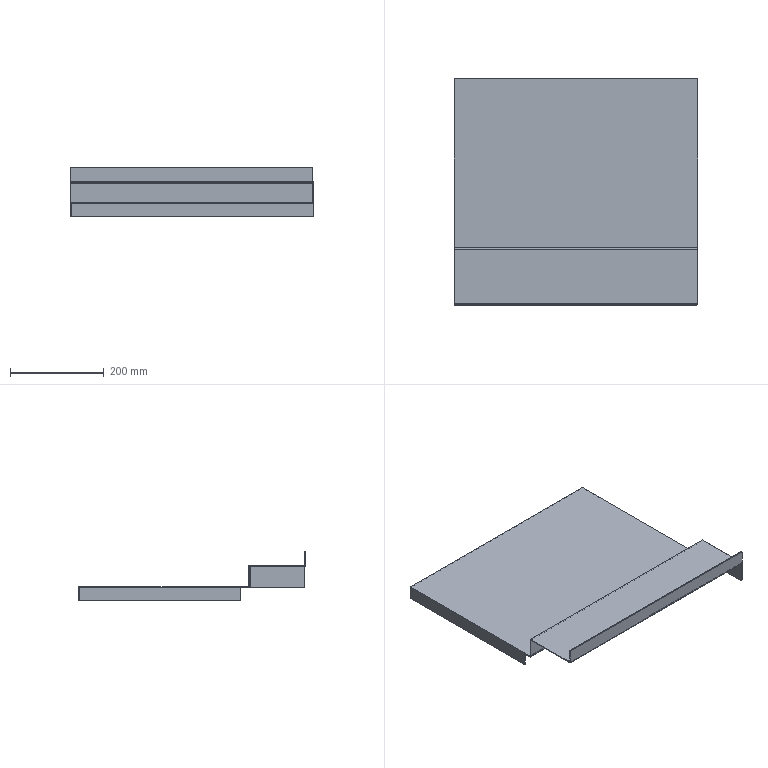Part | STEP file | 11-GYJJ-012-q111 | 1 solid | 31 faces | box 521 x 485 x 105 mm | volume 642321 mm3 | plane 21 | cylinder 10 | commonest cylinder face diameters 4 x10
STEP:
#1=CARTESIAN_POINT('',(258.5,-300.5,45.));
#2=VERTEX_POINT('',#1);
#3=CARTESIAN_POINT('',(258.5,-184.5,45.));
#4=VERTEX_POINT('',#3);
#5=CARTESIAN_POINT('',(258.5,-184.5,45.));
#6=DIRECTION('',(0.,1.,0.));
#7=VECTOR('',#6,1000.);
#8=LINE('',#5,#7);
#9=EDGE_CURVE('',#2,#4,#8,.T.);
#10=ORIENTED_EDGE('',*,*,#9,.F.);
#11=CARTESIAN_POINT('',(-260.5,-300.5,45.));
#12=VERTEX_POINT('',#11);
#13=CARTESIAN_POINT('',(-260.5,-300.5,45.));
#14=DIRECTION('',(-1.,0.,0.));
#15=VECTOR('',#14,1000.);
#16=LINE('',#13,#15);
#17=EDGE_CURVE('',#2,#12,#16,.T.);
#18=ORIENTED_EDGE('',*,*,#17,.T.);
#19=CARTESIAN_POINT('',(-260.5,-184.5,45.));
#20=VERTEX_POINT('',#19);
#21=CARTESIAN_POINT('',(-260.5,-302.5,45.));
#22=DIRECTION('',(0.,1.,0.));
#23=VECTOR('',#22,1000.);
#24=LINE('',#21,#23);
#25=EDGE_CURVE('',#12,#20,#24,.T.);
#26=ORIENTED_EDGE('',*,*,#25,.T.);
#27=CARTESIAN_POINT('',(260.5,-184.5,45.));
#28=DIRECTION('',(1.,0.,0.));
#29=VECTOR('',#28,1000.);
#30=LINE('',#27,#29);
#31=EDGE_CURVE('',#20,#4,#30,.T.);
#32=ORIENTED_EDGE('',*,*,#31,.T.);
#33=EDGE_LOOP('',(#10,#18,#26,#32));
#34=FACE_OUTER_BOUND('',#33,.T.);
#35=CARTESIAN_POINT('',(-260.5,-302.5,45.));
#36=DIRECTION('',(0.,0.,1.));
#37=DIRECTION('',(1.,0.,0.));
#38=AXIS2_PLACEMENT_3D('',#35,#36,#37);
#39=PLANE('',#38);
#40=ADVANCED_FACE('',(#34),#39,.F.);
#41=CARTESIAN_POINT('',(-260.5,-182.5,47.));
#42=VERTEX_POINT('',#41);
#43=CARTESIAN_POINT('',(-260.5,-298.5,47.));
#44=VERTEX_POINT('',#43);
#45=CARTESIAN_POINT('',(-260.5,-182.5,47.));
#46=DIRECTION('',(0.,-1.,0.));
#47=VECTOR('',#46,1000.);
#48=LINE('',#45,#47);
#49=EDGE_CURVE('',#42,#44,#48,.T.);
#50=ORIENTED_EDGE('',*,*,#49,.T.);
#51=CARTESIAN_POINT('',(258.5,-298.5,47.));
#52=VERTEX_POINT('',#51);
#53=CARTESIAN_POINT('',(260.5,-298.5,47.));
#54=DIRECTION('',(1.,0.,0.));
#55=VECTOR('',#54,1000.);
#56=LINE('',#53,#55);
#57=EDGE_CURVE('',#44,#52,#56,.T.);
#58=ORIENTED_EDGE('',*,*,#57,.T.);
#59=CARTESIAN_POINT('',(258.5,-300.5,47.));
#60=VERTEX_POINT('',#59);
#61=CARTESIAN_POINT('',(258.5,-298.5,47.));
#62=DIRECTION('',(0.,1.,0.));
#63=VECTOR('',#62,1000.);
#64=LINE('',#61,#63);
#65=EDGE_CURVE('',#60,#52,#64,.T.);
#66=ORIENTED_EDGE('',*,*,#65,.F.);
#67=CARTESIAN_POINT('',(260.5,-300.5,47.));
#68=VERTEX_POINT('',#67);
#69=CARTESIAN_POINT('',(255.672,-300.5,47.));
#70=DIRECTION('',(1.,0.,0.));
#71=VECTOR('',#70,1000.);
#72=LINE('',#69,#71);
#73=EDGE_CURVE('',#60,#68,#72,.T.);
#74=ORIENTED_EDGE('',*,*,#73,.T.);
#75=CARTESIAN_POINT('',(260.5,-182.5,47.));
#76=VERTEX_POINT('',#75);
#77=CARTESIAN_POINT('',(260.5,-182.5,47.));
#78=DIRECTION('',(0.,1.,0.));
#79=VECTOR('',#78,1000.);
#80=LINE('',#77,#79);
#81=EDGE_CURVE('',#68,#76,#80,.T.);
#82=ORIENTED_EDGE('',*,*,#81,.T.);
#83=CARTESIAN_POINT('',(0.,-182.5,47.));
#84=DIRECTION('',(-1.,0.,0.));
#85=VECTOR('',#84,1000.);
#86=LINE('',#83,#85);
#87=EDGE_CURVE('',#76,#42,#86,.T.);
#88=ORIENTED_EDGE('',*,*,#87,.T.);
#89=EDGE_LOOP('',(#50,#58,#66,#74,#82,#88));
#90=FACE_OUTER_BOUND('',#89,.T.);
#91=CARTESIAN_POINT('',(0.,0.,47.));
#92=DIRECTION('',(0.,0.,-1.));
#93=DIRECTION('',(-1.,0.,0.));
#94=AXIS2_PLACEMENT_3D('',#91,#92,#93);
#95=PLANE('',#94);
#96=ADVANCED_FACE('',(#90),#95,.F.);
#97=CARTESIAN_POINT('',(260.5,-182.5,43.));
#98=VERTEX_POINT('',#97);
#99=CARTESIAN_POINT('',(260.5,-182.5,2.));
#100=VERTEX_POINT('',#99);
#101=CARTESIAN_POINT('',(260.5,-182.5,2.));
#102=DIRECTION('',(0.,0.,-1.));
#103=VECTOR('',#102,1000.);
#104=LINE('',#101,#103);
#105=EDGE_CURVE('',#98,#100,#104,.T.);
#106=ORIENTED_EDGE('',*,*,#105,.F.);
#107=CARTESIAN_POINT('',(-260.5,-182.5,43.));
#108=VERTEX_POINT('',#107);
#109=CARTESIAN_POINT('',(-260.5,-182.5,43.));
#110=DIRECTION('',(-1.,0.,0.));
#111=VECTOR('',#110,1000.);
#112=LINE('',#109,#111);
#113=EDGE_CURVE('',#98,#108,#112,.T.);
#114=ORIENTED_EDGE('',*,*,#113,.T.);
#115=CARTESIAN_POINT('',(-260.5,-182.5,2.));
#116=VERTEX_POINT('',#115);
#117=CARTESIAN_POINT('',(-260.5,-182.5,2.));
#118=DIRECTION('',(0.,0.,-1.));
#119=VECTOR('',#118,1000.);
#120=LINE('',#117,#119);
#121=EDGE_CURVE('',#108,#116,#120,.T.);
#122=ORIENTED_EDGE('',*,*,#121,.T.);
#123=CARTESIAN_POINT('',(-260.5,-182.5,2.));
#124=DIRECTION('',(1.,0.,0.));
#125=VECTOR('',#124,1000.);
#126=LINE('',#123,#125);
#127=EDGE_CURVE('',#116,#100,#126,.T.);
#128=ORIENTED_EDGE('',*,*,#127,.T.);
#129=EDGE_LOOP('',(#106,#114,#122,#128));
#130=FACE_OUTER_BOUND('',#129,.T.);
#131=CARTESIAN_POINT('',(-260.5,-182.5,2.));
#132=DIRECTION('',(0.,1.,0.));
#133=DIRECTION('',(0.,0.,1.));
#134=AXIS2_PLACEMENT_3D('',#131,#132,#133);
#135=PLANE('',#134);
#136=ADVANCED_FACE('',(#130),#135,.F.);
#137=CARTESIAN_POINT('',(260.5,-180.5,0.));
#138=VERTEX_POINT('',#137);
#139=CARTESIAN_POINT('',(260.5,180.5,0.));
#140=VERTEX_POINT('',#139);
#141=CARTESIAN_POINT('',(260.5,182.5,0.));
#142=DIRECTION('',(0.,1.,0.));
#143=VECTOR('',#142,1000.);
#144=LINE('',#141,#143);
#145=EDGE_CURVE('',#138,#140,#144,.T.);
#146=ORIENTED_EDGE('',*,*,#145,.F.);
#147=CARTESIAN_POINT('',(-260.5,-180.5,0.));
#148=VERTEX_POINT('',#147);
#149=CARTESIAN_POINT('',(0.,-180.5,0.));
#150=DIRECTION('',(-1.,0.,0.));
#151=VECTOR('',#150,1000.);
#152=LINE('',#149,#151);
#153=EDGE_CURVE('',#138,#148,#152,.T.);
#154=ORIENTED_EDGE('',*,*,#153,.T.);
#155=CARTESIAN_POINT('',(-260.5,-164.5,0.));
#156=VERTEX_POINT('',#155);
#157=CARTESIAN_POINT('',(-260.5,182.5,0.));
#158=DIRECTION('',(0.,-1.,0.));
#159=VECTOR('',#158,1000.);
#160=LINE('',#157,#159);
#161=EDGE_CURVE('',#156,#148,#160,.T.);
#162=ORIENTED_EDGE('',*,*,#161,.F.);
#163=CARTESIAN_POINT('',(-258.5,-164.5,0.));
#164=VERTEX_POINT('',#163);
#165=CARTESIAN_POINT('',(-260.5,-164.5,0.));
#166=DIRECTION('',(-1.,0.,0.));
#167=VECTOR('',#166,1000.);
#168=LINE('',#165,#167);
#169=EDGE_CURVE('',#164,#156,#168,.T.);
#170=ORIENTED_EDGE('',*,*,#169,.F.);
#171=CARTESIAN_POINT('',(-258.5,180.5,0.));
#172=VERTEX_POINT('',#171);
#173=CARTESIAN_POINT('',(-258.5,180.5,0.));
#174=DIRECTION('',(0.,-1.,0.));
#175=VECTOR('',#174,1000.);
#176=LINE('',#173,#175);
#177=EDGE_CURVE('',#172,#164,#176,.T.);
#178=ORIENTED_EDGE('',*,*,#177,.F.);
#179=CARTESIAN_POINT('',(260.5,180.5,0.));
#180=DIRECTION('',(-1.,0.,0.));
#181=VECTOR('',#180,1000.);
#182=LINE('',#179,#181);
#183=EDGE_CURVE('',#140,#172,#182,.T.);
#184=ORIENTED_EDGE('',*,*,#183,.F.);
#185=EDGE_LOOP('',(#146,#154,#162,#170,#178,#184));
#186=FACE_OUTER_BOUND('',#185,.T.);
#187=CARTESIAN_POINT('',(0.,0.,0.));
#188=DIRECTION('',(0.,0.,1.));
#189=DIRECTION('',(1.,0.,0.));
#190=AXIS2_PLACEMENT_3D('',#187,#188,#189);
#191=PLANE('',#190);
#192=ADVANCED_FACE('',(#186),#191,.F.);
#193=CARTESIAN_POINT('',(-258.5,180.5,-28.));
#194=VERTEX_POINT('',#193);
#195=CARTESIAN_POINT('',(-258.5,180.5,-28.));
#196=DIRECTION('',(0.,0.,1.));
#197=VECTOR('',#196,1000.);
#198=LINE('',#195,#197);
#199=EDGE_CURVE('',#194,#172,#198,.T.);
#200=ORIENTED_EDGE('',*,*,#199,.F.);
#201=CARTESIAN_POINT('',(260.5,180.5,-28.));
#202=VERTEX_POINT('',#201);
#203=CARTESIAN_POINT('',(260.5,180.5,-28.));
#204=DIRECTION('',(-1.,0.,0.));
#205=VECTOR('',#204,1000.);
#206=LINE('',#203,#205);
#207=EDGE_CURVE('',#202,#194,#206,.T.);
#208=ORIENTED_EDGE('',*,*,#207,.F.);
#209=CARTESIAN_POINT('',(260.5,180.5,-28.));
#210=DIRECTION('',(0.,0.,1.));
#211=VECTOR('',#210,1000.);
#212=LINE('',#209,#211);
#213=EDGE_CURVE('',#202,#140,#212,.T.);
#214=ORIENTED_EDGE('',*,*,#213,.T.);
#215=ORIENTED_EDGE('',*,*,#183,.T.);
#216=EDGE_LOOP('',(#200,#208,#214,#215));
#217=FACE_OUTER_BOUND('',#216,.T.);
#218=CARTESIAN_POINT('',(260.5,180.5,-28.));
#219=DIRECTION('',(0.,1.,0.));
#220=DIRECTION('',(-1.,0.,0.));
#221=AXIS2_PLACEMENT_3D('',#218,#219,#220);
#222=PLANE('',#221);
#223=ADVANCED_FACE('',(#217),#222,.F.);
#224=CARTESIAN_POINT('',(260.5,-298.5,0.));
#225=VERTEX_POINT('',#224);
#226=CARTESIAN_POINT('',(260.5,-186.5,0.));
#227=VERTEX_POINT('',#226);
#228=CARTESIAN_POINT('',(260.5,-184.5,0.));
#229=DIRECTION('',(0.,1.,0.));
#230=VECTOR('',#229,1000.);
#231=LINE('',#228,#230);
#232=EDGE_CURVE('',#225,#227,#231,.T.);
#233=ORIENTED_EDGE('',*,*,#232,.T.);
#234=CARTESIAN_POINT('',(260.5,-184.5,2.));
#235=VERTEX_POINT('',#234);
#236=CARTESIAN_POINT('',(260.5,-186.5,2.));
#237=DIRECTION('',(1.,0.,0.));
#238=DIRECTION('',(0.,0.,1.));
#239=AXIS2_PLACEMENT_3D('',#236,#237,#238);
#240=CIRCLE('',#239,2.);
#241=EDGE_CURVE('',#227,#235,#240,.T.);
#242=ORIENTED_EDGE('',*,*,#241,.T.);
#243=CARTESIAN_POINT('',(260.5,-184.5,45.));
#244=VERTEX_POINT('',#243);
#245=CARTESIAN_POINT('',(260.5,-184.5,-116.017));
#246=DIRECTION('',(0.,0.,1.));
#247=VECTOR('',#246,1000.);
#248=LINE('',#245,#247);
#249=EDGE_CURVE('',#235,#244,#248,.T.);
#250=ORIENTED_EDGE('',*,*,#249,.T.);
#251=CARTESIAN_POINT('',(260.5,-184.5,43.));
#252=DIRECTION('',(-1.,0.,0.));
#253=DIRECTION('',(0.,0.,1.));
#254=AXIS2_PLACEMENT_3D('',#251,#252,#253);
#255=CIRCLE('',#254,2.);
#256=EDGE_CURVE('',#244,#98,#255,.T.);
#257=ORIENTED_EDGE('',*,*,#256,.T.);
#258=ORIENTED_EDGE('',*,*,#105,.T.);
#259=CARTESIAN_POINT('',(260.5,-180.5,2.));
#260=DIRECTION('',(1.,0.,0.));
#261=DIRECTION('',(0.,0.,1.));
#262=AXIS2_PLACEMENT_3D('',#259,#260,#261);
#263=CIRCLE('',#262,2.);
#264=EDGE_CURVE('',#100,#138,#263,.T.);
#265=ORIENTED_EDGE('',*,*,#264,.T.);
#266=ORIENTED_EDGE('',*,*,#145,.T.);
#267=ORIENTED_EDGE('',*,*,#213,.F.);
#268=CARTESIAN_POINT('',(260.5,182.5,-28.));
#269=VERTEX_POINT('',#268);
#270=CARTESIAN_POINT('',(260.5,182.5,-28.));
#271=DIRECTION('',(0.,-1.,0.));
#272=VECTOR('',#271,1000.);
#273=LINE('',#270,#272);
#274=EDGE_CURVE('',#269,#202,#273,.T.);
#275=ORIENTED_EDGE('',*,*,#274,.F.);
#276=CARTESIAN_POINT('',(260.5,182.5,2.));
#277=VERTEX_POINT('',#276);
#278=CARTESIAN_POINT('',(260.5,182.5,2.));
#279=DIRECTION('',(0.,0.,-1.));
#280=VECTOR('',#279,1000.);
#281=LINE('',#278,#280);
#282=EDGE_CURVE('',#277,#269,#281,.T.);
#283=ORIENTED_EDGE('',*,*,#282,.F.);
#284=CARTESIAN_POINT('',(260.5,-178.5,2.));
#285=VERTEX_POINT('',#284);
#286=CARTESIAN_POINT('',(260.5,182.5,2.));
#287=DIRECTION('',(0.,1.,0.));
#288=VECTOR('',#287,1000.);
#289=LINE('',#286,#288);
#290=EDGE_CURVE('',#285,#277,#289,.T.);
#291=ORIENTED_EDGE('',*,*,#290,.F.);
#292=CARTESIAN_POINT('',(260.5,-180.5,4.));
#293=VERTEX_POINT('',#292);
#294=CARTESIAN_POINT('',(260.5,-178.5,4.));
#295=DIRECTION('',(-1.,0.,0.));
#296=DIRECTION('',(0.,0.,1.));
#297=AXIS2_PLACEMENT_3D('',#294,#295,#296);
#298=CIRCLE('',#297,2.);
#299=EDGE_CURVE('',#285,#293,#298,.T.);
#300=ORIENTED_EDGE('',*,*,#299,.T.);
#301=CARTESIAN_POINT('',(260.5,-180.5,45.));
#302=VERTEX_POINT('',#301);
#303=CARTESIAN_POINT('',(260.5,-180.5,47.));
#304=DIRECTION('',(0.,0.,-1.));
#305=VECTOR('',#304,1000.);
#306=LINE('',#303,#305);
#307=EDGE_CURVE('',#302,#293,#306,.T.);
#308=ORIENTED_EDGE('',*,*,#307,.F.);
#309=CARTESIAN_POINT('',(260.5,-182.5,45.));
#310=DIRECTION('',(1.,0.,0.));
#311=DIRECTION('',(0.,0.,1.));
#312=AXIS2_PLACEMENT_3D('',#309,#310,#311);
#313=CIRCLE('',#312,2.);
#314=EDGE_CURVE('',#302,#76,#313,.T.);
#315=ORIENTED_EDGE('',*,*,#314,.T.);
#316=ORIENTED_EDGE('',*,*,#81,.F.);
#317=CARTESIAN_POINT('',(260.5,-300.5,2.));
#318=VERTEX_POINT('',#317);
#319=CARTESIAN_POINT('',(260.5,-300.5,-116.017));
#320=DIRECTION('',(0.,0.,1.));
#321=VECTOR('',#320,1000.);
#322=LINE('',#319,#321);
#323=EDGE_CURVE('',#318,#68,#322,.T.);
#324=ORIENTED_EDGE('',*,*,#323,.F.);
#325=CARTESIAN_POINT('',(260.5,-298.5,2.));
#326=DIRECTION('',(1.,0.,0.));
#327=DIRECTION('',(0.,0.,1.));
#328=AXIS2_PLACEMENT_3D('',#325,#326,#327);
#329=CIRCLE('',#328,2.);
#330=EDGE_CURVE('',#318,#225,#329,.T.);
#331=ORIENTED_EDGE('',*,*,#330,.T.);
#332=EDGE_LOOP('',(#233,#242,#250,#257,#258,#265,#266,#267,#275,#283,#291,#300,#308,#315,#316,#324,#331));
#333=FACE_OUTER_BOUND('',#332,.T.);
#334=CARTESIAN_POINT('',(260.5,182.5,2.));
#335=DIRECTION('',(-1.,0.,0.));
#336=DIRECTION('',(0.,0.,1.));
#337=AXIS2_PLACEMENT_3D('',#334,#335,#336);
#338=PLANE('',#337);
#339=ADVANCED_FACE('',(#333),#338,.F.);
#340=ORIENTED_EDGE('',*,*,#282,.T.);
#341=CARTESIAN_POINT('',(-260.5,182.5,-28.));
#342=VERTEX_POINT('',#341);
#343=CARTESIAN_POINT('',(260.5,182.5,-28.));
#344=DIRECTION('',(1.,0.,0.));
#345=VECTOR('',#344,1000.);
#346=LINE('',#343,#345);
#347=EDGE_CURVE('',#342,#269,#346,.T.);
#348=ORIENTED_EDGE('',*,*,#347,.F.);
#349=CARTESIAN_POINT('',(-260.5,182.5,2.));
#350=VERTEX_POINT('',#349);
#351=CARTESIAN_POINT('',(-260.5,182.5,2.));
#352=DIRECTION('',(0.,0.,-1.));
#353=VECTOR('',#352,1000.);
#354=LINE('',#351,#353);
#355=EDGE_CURVE('',#350,#342,#354,.T.);
#356=ORIENTED_EDGE('',*,*,#355,.F.);
#357=CARTESIAN_POINT('',(-260.5,182.5,2.));
#358=DIRECTION('',(-1.,0.,0.));
#359=VECTOR('',#358,1000.);
#360=LINE('',#357,#359);
#361=EDGE_CURVE('',#277,#350,#360,.T.);
#362=ORIENTED_EDGE('',*,*,#361,.F.);
#363=EDGE_LOOP('',(#340,#348,#356,#362));
#364=FACE_OUTER_BOUND('',#363,.T.);
#365=CARTESIAN_POINT('',(-260.5,182.5,2.));
#366=DIRECTION('',(0.,-1.,0.));
#367=DIRECTION('',(0.,0.,-1.));
#368=AXIS2_PLACEMENT_3D('',#365,#366,#367);
#369=PLANE('',#368);
#370=ADVANCED_FACE('',(#364),#369,.F.);
#371=CARTESIAN_POINT('',(-260.5,-302.5,75.));
#372=VERTEX_POINT('',#371);
#373=CARTESIAN_POINT('',(-260.5,-302.5,47.));
#374=VERTEX_POINT('',#373);
#375=CARTESIAN_POINT('',(-260.5,-302.5,47.));
#376=DIRECTION('',(0.,0.,-1.));
#377=VECTOR('',#376,1000.);
#378=LINE('',#375,#377);
#379=EDGE_CURVE('',#372,#374,#378,.T.);
#380=ORIENTED_EDGE('',*,*,#379,.F.);
#381=CARTESIAN_POINT('',(-260.5,-300.5,75.));
#382=VERTEX_POINT('',#381);
#383=CARTESIAN_POINT('',(-260.5,182.5,75.));
#384=DIRECTION('',(0.,1.,0.));
#385=VECTOR('',#384,1000.);
#386=LINE('',#383,#385);
#387=EDGE_CURVE('',#372,#382,#386,.T.);
#388=ORIENTED_EDGE('',*,*,#387,.T.);
#389=CARTESIAN_POINT('',(-260.5,-300.5,49.));
#390=VERTEX_POINT('',#389);
#391=CARTESIAN_POINT('',(-260.5,-300.5,77.));
#392=DIRECTION('',(0.,0.,-1.));
#393=VECTOR('',#392,1000.);
#394=LINE('',#391,#393);
#395=EDGE_CURVE('',#382,#390,#394,.T.);
#396=ORIENTED_EDGE('',*,*,#395,.T.);
#397=CARTESIAN_POINT('',(-260.5,-298.5,49.));
#398=DIRECTION('',(1.,0.,0.));
#399=DIRECTION('',(0.,1.,0.));
#400=AXIS2_PLACEMENT_3D('',#397,#398,#399);
#401=CIRCLE('',#400,2.);
#402=EDGE_CURVE('',#390,#44,#401,.T.);
#403=ORIENTED_EDGE('',*,*,#402,.T.);
#404=ORIENTED_EDGE('',*,*,#49,.F.);
#405=CARTESIAN_POINT('',(-260.5,-180.5,45.));
#406=VERTEX_POINT('',#405);
#407=CARTESIAN_POINT('',(-260.5,-182.5,45.));
#408=DIRECTION('',(-1.,0.,0.));
#409=DIRECTION('',(0.,1.,0.));
#410=AXIS2_PLACEMENT_3D('',#407,#408,#409);
#411=CIRCLE('',#410,2.);
#412=EDGE_CURVE('',#42,#406,#411,.T.);
#413=ORIENTED_EDGE('',*,*,#412,.T.);
#414=CARTESIAN_POINT('',(-260.5,-180.5,4.));
#415=VERTEX_POINT('',#414);
#416=CARTESIAN_POINT('',(-260.5,-180.5,47.));
#417=DIRECTION('',(0.,0.,-1.));
#418=VECTOR('',#417,1000.);
#419=LINE('',#416,#418);
#420=EDGE_CURVE('',#406,#415,#419,.T.);
#421=ORIENTED_EDGE('',*,*,#420,.T.);
#422=CARTESIAN_POINT('',(-260.5,-178.5,2.));
#423=VERTEX_POINT('',#422);
#424=CARTESIAN_POINT('',(-260.5,-178.5,4.));
#425=DIRECTION('',(1.,0.,0.));
#426=DIRECTION('',(0.,1.,0.));
#427=AXIS2_PLACEMENT_3D('',#424,#425,#426);
#428=CIRCLE('',#427,2.);
#429=EDGE_CURVE('',#415,#423,#428,.T.);
#430=ORIENTED_EDGE('',*,*,#429,.T.);
#431=CARTESIAN_POINT('',(-260.5,182.5,2.));
#432=DIRECTION('',(0.,-1.,0.));
#433=VECTOR('',#432,1000.);
#434=LINE('',#431,#433);
#435=EDGE_CURVE('',#350,#423,#434,.T.);
#436=ORIENTED_EDGE('',*,*,#435,.F.);
#437=ORIENTED_EDGE('',*,*,#355,.T.);
#438=CARTESIAN_POINT('',(-260.5,-164.5,-28.));
#439=VERTEX_POINT('',#438);
#440=CARTESIAN_POINT('',(-260.5,182.5,-28.));
#441=DIRECTION('',(0.,1.,0.));
#442=VECTOR('',#441,1000.);
#443=LINE('',#440,#442);
#444=EDGE_CURVE('',#439,#342,#443,.T.);
#445=ORIENTED_EDGE('',*,*,#444,.F.);
#446=CARTESIAN_POINT('',(-260.5,-164.5,-28.));
#447=DIRECTION('',(0.,0.,1.));
#448=VECTOR('',#447,1000.);
#449=LINE('',#446,#448);
#450=EDGE_CURVE('',#439,#156,#449,.T.);
#451=ORIENTED_EDGE('',*,*,#450,.T.);
#452=ORIENTED_EDGE('',*,*,#161,.T.);
#453=CARTESIAN_POINT('',(-260.5,-180.5,2.));
#454=DIRECTION('',(-1.,0.,0.));
#455=DIRECTION('',(0.,1.,0.));
#456=AXIS2_PLACEMENT_3D('',#453,#454,#455);
#457=CIRCLE('',#456,2.);
#458=EDGE_CURVE('',#148,#116,#457,.T.);
#459=ORIENTED_EDGE('',*,*,#458,.T.);
#460=ORIENTED_EDGE('',*,*,#121,.F.);
#461=CARTESIAN_POINT('',(-260.5,-184.5,43.));
#462=DIRECTION('',(1.,0.,0.));
#463=DIRECTION('',(0.,1.,0.));
#464=AXIS2_PLACEMENT_3D('',#461,#462,#463);
#465=CIRCLE('',#464,2.);
#466=EDGE_CURVE('',#108,#20,#465,.T.);
#467=ORIENTED_EDGE('',*,*,#466,.T.);
#468=ORIENTED_EDGE('',*,*,#25,.F.);
#469=CARTESIAN_POINT('',(-260.5,-300.5,47.));
#470=DIRECTION('',(-1.,0.,0.));
#471=DIRECTION('',(0.,1.,0.));
#472=AXIS2_PLACEMENT_3D('',#469,#470,#471);
#473=CIRCLE('',#472,2.);
#474=EDGE_CURVE('',#12,#374,#473,.T.);
#475=ORIENTED_EDGE('',*,*,#474,.T.);
#476=EDGE_LOOP('',(#380,#388,#396,#403,#404,#413,#421,#430,#436,#437,#445,#451,#452,#459,#460,#467,#468,#475));
#477=FACE_OUTER_BOUND('',#476,.T.);
#478=CARTESIAN_POINT('',(-260.5,182.5,2.));
#479=DIRECTION('',(1.,0.,0.));
#480=DIRECTION('',(0.,1.,0.));
#481=AXIS2_PLACEMENT_3D('',#478,#479,#480);
#482=PLANE('',#481);
#483=ADVANCED_FACE('',(#477),#482,.F.);
#484=ORIENTED_EDGE('',*,*,#435,.T.);
#485=CARTESIAN_POINT('',(0.,-178.5,2.));
#486=DIRECTION('',(1.,0.,0.));
#487=VECTOR('',#486,1000.);
#488=LINE('',#485,#487);
#489=EDGE_CURVE('',#423,#285,#488,.T.);
#490=ORIENTED_EDGE('',*,*,#489,.T.);
#491=ORIENTED_EDGE('',*,*,#290,.T.);
#492=ORIENTED_EDGE('',*,*,#361,.T.);
#493=EDGE_LOOP('',(#484,#490,#491,#492));
#494=FACE_OUTER_BOUND('',#493,.T.);
#495=CARTESIAN_POINT('',(0.,0.,2.));
#496=DIRECTION('',(0.,0.,1.));
#497=DIRECTION('',(1.,0.,0.));
#498=AXIS2_PLACEMENT_3D('',#495,#496,#497);
#499=PLANE('',#498);
#500=ADVANCED_FACE('',(#494),#499,.T.);
#501=ORIENTED_EDGE('',*,*,#274,.T.);
#502=ORIENTED_EDGE('',*,*,#207,.T.);
#503=CARTESIAN_POINT('',(-258.5,-164.5,-28.));
#504=VERTEX_POINT('',#503);
#505=CARTESIAN_POINT('',(-258.5,180.5,-28.));
#506=DIRECTION('',(0.,-1.,0.));
#507=VECTOR('',#506,1000.);
#508=LINE('',#505,#507);
#509=EDGE_CURVE('',#194,#504,#508,.T.);
#510=ORIENTED_EDGE('',*,*,#509,.T.);
#511=CARTESIAN_POINT('',(-260.5,-164.5,-28.));
#512=DIRECTION('',(-1.,0.,0.));
#513=VECTOR('',#512,1000.);
#514=LINE('',#511,#513);
#515=EDGE_CURVE('',#504,#439,#514,.T.);
#516=ORIENTED_EDGE('',*,*,#515,.T.);
#517=ORIENTED_EDGE('',*,*,#444,.T.);
#518=ORIENTED_EDGE('',*,*,#347,.T.);
#519=EDGE_LOOP('',(#501,#502,#510,#516,#517,#518));
#520=FACE_OUTER_BOUND('',#519,.T.);
#521=CARTESIAN_POINT('',(0.,0.,-28.));
#522=DIRECTION('',(0.,0.,-1.));
#523=DIRECTION('',(-1.,0.,0.));
#524=AXIS2_PLACEMENT_3D('',#521,#522,#523);
#525=PLANE('',#524);
#526=ADVANCED_FACE('',(#520),#525,.T.);
#527=ORIENTED_EDGE('',*,*,#177,.T.);
#528=CARTESIAN_POINT('',(-258.5,-164.5,-28.));
#529=DIRECTION('',(0.,0.,1.));
#530=VECTOR('',#529,1000.);
#531=LINE('',#528,#530);
#532=EDGE_CURVE('',#504,#164,#531,.T.);
#533=ORIENTED_EDGE('',*,*,#532,.F.);
#534=ORIENTED_EDGE('',*,*,#509,.F.);
#535=ORIENTED_EDGE('',*,*,#199,.T.);
#536=EDGE_LOOP('',(#527,#533,#534,#535));
#537=FACE_OUTER_BOUND('',#536,.T.);
#538=CARTESIAN_POINT('',(-258.5,180.5,-28.));
#539=DIRECTION('',(-1.,0.,0.));
#540=DIRECTION('',(0.,-1.,0.));
#541=AXIS2_PLACEMENT_3D('',#538,#539,#540);
#542=PLANE('',#541);
#543=ADVANCED_FACE('',(#537),#542,.F.);
#544=ORIENTED_EDGE('',*,*,#169,.T.);
#545=ORIENTED_EDGE('',*,*,#450,.F.);
#546=ORIENTED_EDGE('',*,*,#515,.F.);
#547=ORIENTED_EDGE('',*,*,#532,.T.);
#548=EDGE_LOOP('',(#544,#545,#546,#547));
#549=FACE_OUTER_BOUND('',#548,.T.);
#550=CARTESIAN_POINT('',(-260.5,-164.5,-28.));
#551=DIRECTION('',(0.,1.,0.));
#552=DIRECTION('',(0.,0.,1.));
#553=AXIS2_PLACEMENT_3D('',#550,#551,#552);
#554=PLANE('',#553);
#555=ADVANCED_FACE('',(#549),#554,.F.);
#556=ORIENTED_EDGE('',*,*,#420,.F.);
#557=CARTESIAN_POINT('',(-260.5,-180.5,45.));
#558=DIRECTION('',(1.,0.,0.));
#559=VECTOR('',#558,1000.);
#560=LINE('',#557,#559);
#561=EDGE_CURVE('',#406,#302,#560,.T.);
#562=ORIENTED_EDGE('',*,*,#561,.T.);
#563=ORIENTED_EDGE('',*,*,#307,.T.);
#564=CARTESIAN_POINT('',(-260.5,-180.5,4.));
#565=DIRECTION('',(-1.,0.,0.));
#566=VECTOR('',#565,1000.);
#567=LINE('',#564,#566);
#568=EDGE_CURVE('',#293,#415,#567,.T.);
#569=ORIENTED_EDGE('',*,*,#568,.T.);
#570=EDGE_LOOP('',(#556,#562,#563,#569));
#571=FACE_OUTER_BOUND('',#570,.T.);
#572=CARTESIAN_POINT('',(-260.5,-180.5,47.));
#573=DIRECTION('',(0.,-1.,0.));
#574=DIRECTION('',(0.,0.,-1.));
#575=AXIS2_PLACEMENT_3D('',#572,#573,#574);
#576=PLANE('',#575);
#577=ADVANCED_FACE('',(#571),#576,.F.);
#578=CARTESIAN_POINT('',(-258.5,-302.5,77.));
#579=VERTEX_POINT('',#578);
#580=CARTESIAN_POINT('',(256.5,-302.5,77.));
#581=VERTEX_POINT('',#580);
#582=CARTESIAN_POINT('',(-260.5,-302.5,77.));
#583=DIRECTION('',(1.,0.,0.));
#584=VECTOR('',#583,1000.);
#585=LINE('',#582,#584);
#586=EDGE_CURVE('',#579,#581,#585,.T.);
#587=ORIENTED_EDGE('',*,*,#586,.F.);
#588=CARTESIAN_POINT('',(-258.5,-302.5,75.));
#589=DIRECTION('',(0.,-1.,0.));
#590=DIRECTION('',(0.,0.,-1.));
#591=AXIS2_PLACEMENT_3D('',#588,#589,#590);
#592=CIRCLE('',#591,2.);
#593=EDGE_CURVE('',#579,#372,#592,.T.);
#594=ORIENTED_EDGE('',*,*,#593,.T.);
#595=ORIENTED_EDGE('',*,*,#379,.T.);
#596=CARTESIAN_POINT('',(258.5,-302.5,47.));
#597=VERTEX_POINT('',#596);
#598=CARTESIAN_POINT('',(260.5,-302.5,47.));
#599=DIRECTION('',(1.,0.,0.));
#600=VECTOR('',#599,1000.);
#601=LINE('',#598,#600);
#602=EDGE_CURVE('',#374,#597,#601,.T.);
#603=ORIENTED_EDGE('',*,*,#602,.T.);
#604=CARTESIAN_POINT('',(258.5,-302.5,75.));
#605=VERTEX_POINT('',#604);
#606=CARTESIAN_POINT('',(258.5,-302.5,77.));
#607=DIRECTION('',(0.,0.,-1.));
#608=VECTOR('',#607,1000.);
#609=LINE('',#606,#608);
#610=EDGE_CURVE('',#605,#597,#609,.T.);
#611=ORIENTED_EDGE('',*,*,#610,.F.);
#612=CARTESIAN_POINT('',(256.5,-302.5,75.));
#613=DIRECTION('',(0.,-1.,0.));
#614=DIRECTION('',(0.,0.,-1.));
#615=AXIS2_PLACEMENT_3D('',#612,#613,#614);
#616=CIRCLE('',#615,2.);
#617=EDGE_CURVE('',#605,#581,#616,.T.);
#618=ORIENTED_EDGE('',*,*,#617,.T.);
#619=EDGE_LOOP('',(#587,#594,#595,#603,#611,#618));
#620=FACE_OUTER_BOUND('',#619,.T.);
#621=CARTESIAN_POINT('',(0.,-302.5,0.));
#622=DIRECTION('',(0.,-1.,0.));
#623=DIRECTION('',(0.,0.,-1.));
#624=AXIS2_PLACEMENT_3D('',#621,#622,#623);
#625=PLANE('',#624);
#626=ADVANCED_FACE('',(#620),#625,.T.);
#627=ORIENTED_EDGE('',*,*,#395,.F.);
#628=CARTESIAN_POINT('',(-258.5,-300.5,77.));
#629=VERTEX_POINT('',#628);
#630=CARTESIAN_POINT('',(-258.5,-300.5,75.));
#631=DIRECTION('',(0.,1.,0.));
#632=DIRECTION('',(0.,0.,-1.));
#633=AXIS2_PLACEMENT_3D('',#630,#631,#632);
#634=CIRCLE('',#633,2.);
#635=EDGE_CURVE('',#382,#629,#634,.T.);
#636=ORIENTED_EDGE('',*,*,#635,.T.);
#637=CARTESIAN_POINT('',(256.5,-300.5,77.));
#638=VERTEX_POINT('',#637);
#639=CARTESIAN_POINT('',(-260.5,-300.5,77.));
#640=DIRECTION('',(-1.,0.,0.));
#641=VECTOR('',#640,1000.);
#642=LINE('',#639,#641);
#643=EDGE_CURVE('',#638,#629,#642,.T.);
#644=ORIENTED_EDGE('',*,*,#643,.F.);
#645=CARTESIAN_POINT('',(258.5,-300.5,75.));
#646=VERTEX_POINT('',#645);
#647=CARTESIAN_POINT('',(256.5,-300.5,75.));
#648=DIRECTION('',(0.,1.,0.));
#649=DIRECTION('',(0.,0.,-1.));
#650=AXIS2_PLACEMENT_3D('',#647,#648,#649);
#651=CIRCLE('',#650,2.);
#652=EDGE_CURVE('',#638,#646,#651,.T.);
#653=ORIENTED_EDGE('',*,*,#652,.T.);
#654=CARTESIAN_POINT('',(258.5,-300.5,49.));
#655=VERTEX_POINT('',#654);
#656=CARTESIAN_POINT('',(258.5,-300.5,77.));
#657=DIRECTION('',(0.,0.,-1.));
#658=VECTOR('',#657,1000.);
#659=LINE('',#656,#658);
#660=EDGE_CURVE('',#646,#655,#659,.T.);
#661=ORIENTED_EDGE('',*,*,#660,.T.);
#662=CARTESIAN_POINT('',(-260.5,-300.5,49.));
#663=DIRECTION('',(-1.,0.,0.));
#664=VECTOR('',#663,1000.);
#665=LINE('',#662,#664);
#666=EDGE_CURVE('',#655,#390,#665,.T.);
#667=ORIENTED_EDGE('',*,*,#666,.T.);
#668=EDGE_LOOP('',(#627,#636,#644,#653,#661,#667));
#669=FACE_OUTER_BOUND('',#668,.T.);
#670=CARTESIAN_POINT('',(-260.5,-300.5,77.));
#671=DIRECTION('',(0.,-1.,0.));
#672=DIRECTION('',(0.,0.,-1.));
#673=AXIS2_PLACEMENT_3D('',#670,#671,#672);
#674=PLANE('',#673);
#675=ADVANCED_FACE('',(#669),#674,.F.);
#676=ORIENTED_EDGE('',*,*,#643,.T.);
#677=CARTESIAN_POINT('',(-258.5,0.,77.));
#678=DIRECTION('',(0.,-1.,0.));
#679=VECTOR('',#678,1000.);
#680=LINE('',#677,#679);
#681=EDGE_CURVE('',#629,#579,#680,.T.);
#682=ORIENTED_EDGE('',*,*,#681,.T.);
#683=ORIENTED_EDGE('',*,*,#586,.T.);
#684=CARTESIAN_POINT('',(256.5,0.,77.));
#685=DIRECTION('',(0.,1.,0.));
#686=VECTOR('',#685,1000.);
#687=LINE('',#684,#686);
#688=EDGE_CURVE('',#581,#638,#687,.T.);
#689=ORIENTED_EDGE('',*,*,#688,.T.);
#690=EDGE_LOOP('',(#676,#682,#683,#689));
#691=FACE_OUTER_BOUND('',#690,.T.);
#692=CARTESIAN_POINT('',(0.,0.,77.));
#693=DIRECTION('',(0.,0.,-1.));
#694=DIRECTION('',(-1.,0.,0.));
#695=AXIS2_PLACEMENT_3D('',#692,#693,#694);
#696=PLANE('',#695);
#697=ADVANCED_FACE('',(#691),#696,.F.);
#698=ORIENTED_EDGE('',*,*,#666,.F.);
#699=CARTESIAN_POINT('',(258.5,-298.5,49.));
#700=DIRECTION('',(1.,0.,0.));
#701=DIRECTION('',(0.,0.,1.));
#702=AXIS2_PLACEMENT_3D('',#699,#700,#701);
#703=CIRCLE('',#702,2.);
#704=EDGE_CURVE('',#655,#52,#703,.T.);
#705=ORIENTED_EDGE('',*,*,#704,.T.);
#706=ORIENTED_EDGE('',*,*,#57,.F.);
#707=ORIENTED_EDGE('',*,*,#402,.F.);
#708=EDGE_LOOP('',(#698,#705,#706,#707));
#709=FACE_OUTER_BOUND('',#708,.T.);
#710=CARTESIAN_POINT('',(-260.5,-298.5,49.));
#711=DIRECTION('',(1.,0.,0.));
#712=DIRECTION('',(0.,0.,-1.));
#713=AXIS2_PLACEMENT_3D('',#710,#711,#712);
#714=CYLINDRICAL_SURFACE('',#713,2.);
#715=ADVANCED_FACE('',(#709),#714,.F.);
#716=CARTESIAN_POINT('',(258.5,-300.5,47.));
#717=DIRECTION('',(1.,0.,0.));
#718=DIRECTION('',(0.,0.,1.));
#719=AXIS2_PLACEMENT_3D('',#716,#717,#718);
#720=CIRCLE('',#719,2.);
#721=EDGE_CURVE('',#597,#2,#720,.T.);
#722=ORIENTED_EDGE('',*,*,#721,.F.);
#723=ORIENTED_EDGE('',*,*,#602,.F.);
#724=ORIENTED_EDGE('',*,*,#474,.F.);
#725=ORIENTED_EDGE('',*,*,#17,.F.);
#726=EDGE_LOOP('',(#722,#723,#724,#725));
#727=FACE_OUTER_BOUND('',#726,.T.);
#728=CARTESIAN_POINT('',(0.,-300.5,47.));
#729=DIRECTION('',(-1.,0.,0.));
#730=DIRECTION('',(0.,0.,1.));
#731=AXIS2_PLACEMENT_3D('',#728,#729,#730);
#732=CYLINDRICAL_SURFACE('',#731,2.);
#733=ADVANCED_FACE('',(#727),#732,.T.);
#734=ORIENTED_EDGE('',*,*,#466,.F.);
#735=ORIENTED_EDGE('',*,*,#113,.F.);
#736=ORIENTED_EDGE('',*,*,#256,.F.);
#737=CARTESIAN_POINT('',(260.5,-184.5,45.));
#738=DIRECTION('',(1.,0.,0.));
#739=VECTOR('',#738,1000.);
#740=LINE('',#737,#739);
#741=EDGE_CURVE('',#4,#244,#740,.T.);
#742=ORIENTED_EDGE('',*,*,#741,.F.);
#743=ORIENTED_EDGE('',*,*,#31,.F.);
#744=EDGE_LOOP('',(#734,#735,#736,#742,#743));
#745=FACE_OUTER_BOUND('',#744,.T.);
#746=CARTESIAN_POINT('',(-260.5,-184.5,43.));
#747=DIRECTION('',(-1.,0.,0.));
#748=DIRECTION('',(0.,0.,1.));
#749=AXIS2_PLACEMENT_3D('',#746,#747,#748);
#750=CYLINDRICAL_SURFACE('',#749,2.);
#751=ADVANCED_FACE('',(#745),#750,.F.);
#752=ORIENTED_EDGE('',*,*,#314,.F.);
#753=ORIENTED_EDGE('',*,*,#561,.F.);
#754=ORIENTED_EDGE('',*,*,#412,.F.);
#755=ORIENTED_EDGE('',*,*,#87,.F.);
#756=EDGE_LOOP('',(#752,#753,#754,#755));
#757=FACE_OUTER_BOUND('',#756,.T.);
#758=CARTESIAN_POINT('',(0.,-182.5,45.));
#759=DIRECTION('',(-1.,0.,0.));
#760=DIRECTION('',(0.,0.,1.));
#761=AXIS2_PLACEMENT_3D('',#758,#759,#760);
#762=CYLINDRICAL_SURFACE('',#761,2.);
#763=ADVANCED_FACE('',(#757),#762,.T.);
#764=ORIENTED_EDGE('',*,*,#299,.F.);
#765=ORIENTED_EDGE('',*,*,#489,.F.);
#766=ORIENTED_EDGE('',*,*,#429,.F.);
#767=ORIENTED_EDGE('',*,*,#568,.F.);
#768=EDGE_LOOP('',(#764,#765,#766,#767));
#769=FACE_OUTER_BOUND('',#768,.T.);
#770=CARTESIAN_POINT('',(-260.5,-178.5,4.));
#771=DIRECTION('',(-1.,0.,0.));
#772=DIRECTION('',(0.,0.,1.));
#773=AXIS2_PLACEMENT_3D('',#770,#771,#772);
#774=CYLINDRICAL_SURFACE('',#773,2.);
#775=ADVANCED_FACE('',(#769),#774,.F.);
#776=ORIENTED_EDGE('',*,*,#458,.F.);
#777=ORIENTED_EDGE('',*,*,#153,.F.);
#778=ORIENTED_EDGE('',*,*,#264,.F.);
#779=ORIENTED_EDGE('',*,*,#127,.F.);
#780=EDGE_LOOP('',(#776,#777,#778,#779));
#781=FACE_OUTER_BOUND('',#780,.T.);
#782=CARTESIAN_POINT('',(-260.5,-180.5,2.));
#783=DIRECTION('',(1.,0.,0.));
#784=DIRECTION('',(0.,0.,-1.));
#785=AXIS2_PLACEMENT_3D('',#782,#783,#784);
#786=CYLINDRICAL_SURFACE('',#785,2.);
#787=ADVANCED_FACE('',(#781),#786,.T.);
#788=ORIENTED_EDGE('',*,*,#249,.F.);
#789=CARTESIAN_POINT('',(258.5,-184.5,2.));
#790=VERTEX_POINT('',#789);
#791=CARTESIAN_POINT('',(260.5,-184.5,2.));
#792=DIRECTION('',(-1.,0.,0.));
#793=VECTOR('',#792,1000.);
#794=LINE('',#791,#793);
#795=EDGE_CURVE('',#235,#790,#794,.T.);
#796=ORIENTED_EDGE('',*,*,#795,.T.);
#797=CARTESIAN_POINT('',(258.5,-184.5,-116.017));
#798=DIRECTION('',(0.,0.,1.));
#799=VECTOR('',#798,1000.);
#800=LINE('',#797,#799);
#801=EDGE_CURVE('',#790,#4,#800,.T.);
#802=ORIENTED_EDGE('',*,*,#801,.T.);
#803=ORIENTED_EDGE('',*,*,#741,.T.);
#804=EDGE_LOOP('',(#788,#796,#802,#803));
#805=FACE_OUTER_BOUND('',#804,.T.);
#806=CARTESIAN_POINT('',(260.5,-184.5,-116.017));
#807=DIRECTION('',(0.,-1.,0.));
#808=DIRECTION('',(0.,0.,-1.));
#809=AXIS2_PLACEMENT_3D('',#806,#807,#808);
#810=PLANE('',#809);
#811=ADVANCED_FACE('',(#805),#810,.F.);
#812=ORIENTED_EDGE('',*,*,#801,.F.);
#813=CARTESIAN_POINT('',(258.5,-186.5,0.));
#814=VERTEX_POINT('',#813);
#815=CARTESIAN_POINT('',(258.5,-186.5,2.));
#816=DIRECTION('',(-1.,0.,0.));
#817=DIRECTION('',(0.,1.,0.));
#818=AXIS2_PLACEMENT_3D('',#815,#816,#817);
#819=CIRCLE('',#818,2.);
#820=EDGE_CURVE('',#790,#814,#819,.T.);
#821=ORIENTED_EDGE('',*,*,#820,.T.);
#822=CARTESIAN_POINT('',(258.5,-298.5,0.));
#823=VERTEX_POINT('',#822);
#824=CARTESIAN_POINT('',(258.5,-184.5,0.));
#825=DIRECTION('',(0.,-1.,0.));
#826=VECTOR('',#825,1000.);
#827=LINE('',#824,#826);
#828=EDGE_CURVE('',#814,#823,#827,.T.);
#829=ORIENTED_EDGE('',*,*,#828,.T.);
#830=CARTESIAN_POINT('',(258.5,-300.5,2.));
#831=VERTEX_POINT('',#830);
#832=CARTESIAN_POINT('',(258.5,-298.5,2.));
#833=DIRECTION('',(-1.,0.,0.));
#834=DIRECTION('',(0.,1.,0.));
#835=AXIS2_PLACEMENT_3D('',#832,#833,#834);
#836=CIRCLE('',#835,2.);
#837=EDGE_CURVE('',#823,#831,#836,.T.);
#838=ORIENTED_EDGE('',*,*,#837,.T.);
#839=CARTESIAN_POINT('',(258.5,-300.5,-116.017));
#840=DIRECTION('',(0.,0.,1.));
#841=VECTOR('',#840,1000.);
#842=LINE('',#839,#841);
#843=EDGE_CURVE('',#831,#2,#842,.T.);
#844=ORIENTED_EDGE('',*,*,#843,.T.);
#845=ORIENTED_EDGE('',*,*,#9,.T.);
#846=EDGE_LOOP('',(#812,#821,#829,#838,#844,#845));
#847=FACE_OUTER_BOUND('',#846,.T.);
#848=CARTESIAN_POINT('',(258.5,-184.5,-116.017));
#849=DIRECTION('',(1.,0.,0.));
#850=DIRECTION('',(0.,1.,0.));
#851=AXIS2_PLACEMENT_3D('',#848,#849,#850);
#852=PLANE('',#851);
#853=ADVANCED_FACE('',(#847),#852,.F.);
#854=ORIENTED_EDGE('',*,*,#843,.F.);
#855=CARTESIAN_POINT('',(260.5,-300.5,2.));
#856=DIRECTION('',(1.,0.,0.));
#857=VECTOR('',#856,1000.);
#858=LINE('',#855,#857);
#859=EDGE_CURVE('',#831,#318,#858,.T.);
#860=ORIENTED_EDGE('',*,*,#859,.T.);
#861=ORIENTED_EDGE('',*,*,#323,.T.);
#862=ORIENTED_EDGE('',*,*,#73,.F.);
#863=CARTESIAN_POINT('',(258.5,-300.5,77.));
#864=DIRECTION('',(0.,0.,-1.));
#865=VECTOR('',#864,1000.);
#866=LINE('',#863,#865);
#867=EDGE_CURVE('',#60,#2,#866,.T.);
#868=ORIENTED_EDGE('',*,*,#867,.T.);
#869=EDGE_LOOP('',(#854,#860,#861,#862,#868));
#870=FACE_OUTER_BOUND('',#869,.T.);
#871=CARTESIAN_POINT('',(260.5,-300.5,-116.017));
#872=DIRECTION('',(0.,1.,0.));
#873=DIRECTION('',(0.,0.,1.));
#874=AXIS2_PLACEMENT_3D('',#871,#872,#873);
#875=PLANE('',#874);
#876=ADVANCED_FACE('',(#870),#875,.F.);
#877=ORIENTED_EDGE('',*,*,#828,.F.);
#878=CARTESIAN_POINT('',(0.,-186.5,0.));
#879=DIRECTION('',(1.,0.,0.));
#880=VECTOR('',#879,1000.);
#881=LINE('',#878,#880);
#882=EDGE_CURVE('',#814,#227,#881,.T.);
#883=ORIENTED_EDGE('',*,*,#882,.T.);
#884=ORIENTED_EDGE('',*,*,#232,.F.);
#885=CARTESIAN_POINT('',(0.,-298.5,0.));
#886=DIRECTION('',(-1.,0.,0.));
#887=VECTOR('',#886,1000.);
#888=LINE('',#885,#887);
#889=EDGE_CURVE('',#225,#823,#888,.T.);
#890=ORIENTED_EDGE('',*,*,#889,.T.);
#891=EDGE_LOOP('',(#877,#883,#884,#890));
#892=FACE_OUTER_BOUND('',#891,.T.);
#893=CARTESIAN_POINT('',(0.,0.,0.));
#894=DIRECTION('',(0.,0.,1.));
#895=DIRECTION('',(1.,0.,0.));
#896=AXIS2_PLACEMENT_3D('',#893,#894,#895);
#897=PLANE('',#896);
#898=ADVANCED_FACE('',(#892),#897,.F.);
#899=ORIENTED_EDGE('',*,*,#660,.F.);
#900=CARTESIAN_POINT('',(258.5,-300.5,75.));
#901=DIRECTION('',(0.,-1.,0.));
#902=VECTOR('',#901,1000.);
#903=LINE('',#900,#902);
#904=EDGE_CURVE('',#646,#605,#903,.T.);
#905=ORIENTED_EDGE('',*,*,#904,.T.);
#906=ORIENTED_EDGE('',*,*,#610,.T.);
#907=ORIENTED_EDGE('',*,*,#721,.T.);
#908=ORIENTED_EDGE('',*,*,#867,.F.);
#909=ORIENTED_EDGE('',*,*,#65,.T.);
#910=ORIENTED_EDGE('',*,*,#704,.F.);
#911=EDGE_LOOP('',(#899,#905,#906,#907,#908,#909,#910));
#912=FACE_OUTER_BOUND('',#911,.T.);
#913=CARTESIAN_POINT('',(258.5,-300.5,77.));
#914=DIRECTION('',(-1.,0.,0.));
#915=DIRECTION('',(0.,0.,1.));
#916=AXIS2_PLACEMENT_3D('',#913,#914,#915);
#917=PLANE('',#916);
#918=ADVANCED_FACE('',(#912),#917,.F.);
#919=ORIENTED_EDGE('',*,*,#241,.F.);
#920=ORIENTED_EDGE('',*,*,#882,.F.);
#921=ORIENTED_EDGE('',*,*,#820,.F.);
#922=ORIENTED_EDGE('',*,*,#795,.F.);
#923=EDGE_LOOP('',(#919,#920,#921,#922));
#924=FACE_OUTER_BOUND('',#923,.T.);
#925=CARTESIAN_POINT('',(260.5,-186.5,2.));
#926=DIRECTION('',(-1.,0.,0.));
#927=DIRECTION('',(0.,0.,1.));
#928=AXIS2_PLACEMENT_3D('',#925,#926,#927);
#929=CYLINDRICAL_SURFACE('',#928,2.);
#930=ADVANCED_FACE('',(#924),#929,.T.);
#931=ORIENTED_EDGE('',*,*,#837,.F.);
#932=ORIENTED_EDGE('',*,*,#889,.F.);
#933=ORIENTED_EDGE('',*,*,#330,.F.);
#934=ORIENTED_EDGE('',*,*,#859,.F.);
#935=EDGE_LOOP('',(#931,#932,#933,#934));
#936=FACE_OUTER_BOUND('',#935,.T.);
#937=CARTESIAN_POINT('',(260.5,-298.5,2.));
#938=DIRECTION('',(1.,0.,0.));
#939=DIRECTION('',(0.,0.,-1.));
#940=AXIS2_PLACEMENT_3D('',#937,#938,#939);
#941=CYLINDRICAL_SURFACE('',#940,2.);
#942=ADVANCED_FACE('',(#936),#941,.T.);
#943=ORIENTED_EDGE('',*,*,#635,.F.);
#944=ORIENTED_EDGE('',*,*,#387,.F.);
#945=ORIENTED_EDGE('',*,*,#593,.F.);
#946=ORIENTED_EDGE('',*,*,#681,.F.);
#947=EDGE_LOOP('',(#943,#944,#945,#946));
#948=FACE_OUTER_BOUND('',#947,.T.);
#949=CARTESIAN_POINT('',(-258.5,0.,75.));
#950=DIRECTION('',(0.,-1.,0.));
#951=DIRECTION('',(1.,0.,0.));
#952=AXIS2_PLACEMENT_3D('',#949,#950,#951);
#953=CYLINDRICAL_SURFACE('',#952,2.);
#954=ADVANCED_FACE('',(#948),#953,.T.);
#955=ORIENTED_EDGE('',*,*,#652,.F.);
#956=ORIENTED_EDGE('',*,*,#688,.F.);
#957=ORIENTED_EDGE('',*,*,#617,.F.);
#958=ORIENTED_EDGE('',*,*,#904,.F.);
#959=EDGE_LOOP('',(#955,#956,#957,#958));
#960=FACE_OUTER_BOUND('',#959,.T.);
#961=CARTESIAN_POINT('',(256.5,-300.5,75.));
#962=DIRECTION('',(0.,-1.,0.));
#963=DIRECTION('',(0.,0.,-1.));
#964=AXIS2_PLACEMENT_3D('',#961,#962,#963);
#965=CYLINDRICAL_SURFACE('',#964,2.);
#966=ADVANCED_FACE('',(#960),#965,.T.);
#967=CLOSED_SHELL('',(#40,#96,#136,#192,#223,#339,#370,#483,#500,#526,#543,#555,#577,#626,#675,#697,#715,#733,#751,#763,#775,#787,#811,#853,#876,#898,#918,#930,#942,#954,#966));
#968=MANIFOLD_SOLID_BREP('',#967);
#969=CARTESIAN_POINT('',(0.,0.,0.));
#970=DIRECTION('',(0.,0.,1.));
#971=DIRECTION('',(1.,0.,0.));
#972=AXIS2_PLACEMENT_3D('',#969,#970,#971);
#973=(LENGTH_UNIT()NAMED_UNIT(*)SI_UNIT(.MILLI.,.METRE.));
#974=UNCERTAINTY_MEASURE_WITH_UNIT(LENGTH_MEASURE(0.00001),#973,'','');
#975=(NAMED_UNIT(*)PLANE_ANGLE_UNIT()SI_UNIT($,.RADIAN.));
#976=(NAMED_UNIT(*)SI_UNIT($,.STERADIAN.)SOLID_ANGLE_UNIT());
#977=(GEOMETRIC_REPRESENTATION_CONTEXT(3)GLOBAL_UNCERTAINTY_ASSIGNED_CONTEXT((#974))GLOBAL_UNIT_ASSIGNED_CONTEXT((#973,#975,#976))REPRESENTATION_CONTEXT('',''));
#978=ADVANCED_BREP_SHAPE_REPRESENTATION('',(#968,#972),#977);